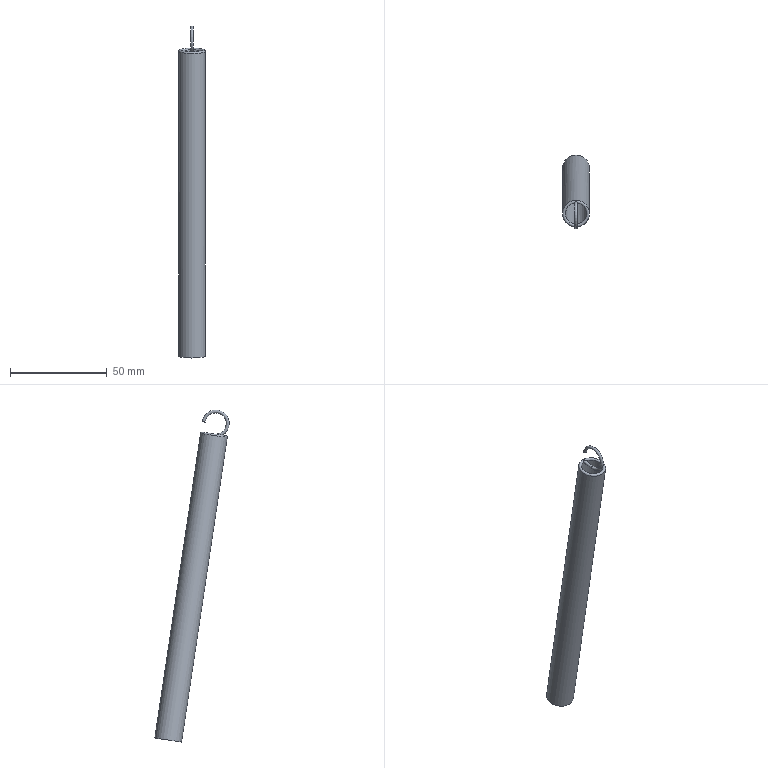Part | NX | features 1 2 | 1 solid | 7 faces | box 14 x 38.473 x 171.94 mm | volume 9491 mm3 | cylinder 3 | plane 2 | torus 2 | commonest cylinder face diameters 1.5 x1 11 x1 14 x1
STEP:
#1=CARTESIAN_POINT('',(-80.065,100.627,-645.601));
#2=VERTEX_POINT('',#1);
#3=CARTESIAN_POINT('',(-80.065,101.371,-645.503));
#4=DIRECTION('',(0.,0.1309,-0.9914));
#5=DIRECTION('',(0.,-0.9914,-0.1309));
#6=AXIS2_PLACEMENT_3D('',#3,#4,#5);
#7=CIRCLE('',#6,0.75);
#8=EDGE_CURVE('',#2,#2,#7,.F.);
#9=ORIENTED_EDGE('',*,*,#8,.F.);
#10=EDGE_LOOP('',(#9));
#11=FACE_BOUND('',#10,.T.);
#12=CARTESIAN_POINT('',(-80.065,101.371,-645.503));
#13=DIRECTION('',(0.,0.1309,-0.9914));
#14=DIRECTION('',(0.,0.9914,0.1309));
#15=AXIS2_PLACEMENT_3D('',#12,#13,#14);
#16=PLANE('',#15);
#17=ADVANCED_FACE('',(#11),#16,.T.);
#18=CARTESIAN_POINT('',(-79.315,96.1,-652.502));
#19=VERTEX_POINT('',#18);
#20=CARTESIAN_POINT('',(-80.065,96.1,-652.502));
#21=DIRECTION('',(0.,0.989,0.1481));
#22=DIRECTION('',(1.,0.,0.));
#23=AXIS2_PLACEMENT_3D('',#20,#21,#22);
#24=CIRCLE('',#23,0.75);
#25=EDGE_CURVE('',#19,#19,#24,.T.);
#26=ORIENTED_EDGE('',*,*,#25,.F.);
#27=EDGE_LOOP('',(#26));
#28=FACE_BOUND('',#27,.T.);
#29=ORIENTED_EDGE('',*,*,#8,.T.);
#30=EDGE_LOOP('',(#29));
#31=FACE_BOUND('',#30,.T.);
#32=CARTESIAN_POINT('',(-80.065,95.174,-646.321));
#33=DIRECTION('',(1.,0.,0.));
#34=DIRECTION('',(0.,-0.989,-0.1481));
#35=AXIS2_PLACEMENT_3D('',#32,#33,#34);
#36=TOROIDAL_SURFACE('',#35,6.25,0.75);
#37=ADVANCED_FACE('',(#28,#31),#36,.T.);
#38=CARTESIAN_POINT('',(-80.065,112.802,-811.261));
#39=VERTEX_POINT('',#38);
#40=CARTESIAN_POINT('',(-80.065,119.725,-810.224));
#41=DIRECTION('',(0.,-0.1481,0.989));
#42=DIRECTION('',(0.,-0.989,-0.1481));
#43=AXIS2_PLACEMENT_3D('',#40,#41,#42);
#44=CIRCLE('',#43,7.);
#45=EDGE_CURVE('',#39,#39,#44,.T.);
#46=ORIENTED_EDGE('',*,*,#45,.T.);
#47=EDGE_LOOP('',(#46));
#48=FACE_BOUND('',#47,.T.);
#49=CARTESIAN_POINT('',(-73.065,96.1,-652.502));
#50=VERTEX_POINT('',#49);
#51=CARTESIAN_POINT('',(-80.065,96.1,-652.502));
#52=DIRECTION('',(0.,0.1481,-0.989));
#53=DIRECTION('',(1.,0.,0.));
#54=AXIS2_PLACEMENT_3D('',#51,#52,#53);
#55=CIRCLE('',#54,7.);
#56=EDGE_CURVE('',#50,#50,#55,.T.);
#57=ORIENTED_EDGE('',*,*,#56,.T.);
#58=EDGE_LOOP('',(#57));
#59=FACE_BOUND('',#58,.T.);
#60=CARTESIAN_POINT('',(-80.065,101.766,-690.33));
#61=DIRECTION('',(0.,0.1481,-0.989));
#62=DIRECTION('',(-1.,0.,0.));
#63=AXIS2_PLACEMENT_3D('',#60,#61,#62);
#64=CYLINDRICAL_SURFACE('',#63,7.);
#65=ADVANCED_FACE('',(#48,#59),#64,.T.);
#66=ORIENTED_EDGE('',*,*,#56,.F.);
#67=EDGE_LOOP('',(#66));
#68=FACE_BOUND('',#67,.T.);
#69=CARTESIAN_POINT('',(-79.315,101.489,-651.695));
#70=VERTEX_POINT('',#69);
#71=CARTESIAN_POINT('',(-80.815,101.489,-651.695));
#72=VERTEX_POINT('',#71);
#73=CARTESIAN_POINT('',(-80.065,96.1,-652.502));
#74=DIRECTION('',(0.,0.1481,-0.989));
#75=DIRECTION('',(-1.,0.,0.));
#76=AXIS2_PLACEMENT_3D('',#73,#74,#75);
#77=CIRCLE('',#76,5.5);
#78=EDGE_CURVE('',#70,#72,#77,.T.);
#79=ORIENTED_EDGE('',*,*,#78,.T.);
#80=CARTESIAN_POINT('',(-80.065,102.17,-650.834));
#81=VERTEX_POINT('',#80);
#82=CARTESIAN_POINT('',(-80.815,101.489,-651.695));
#83=CARTESIAN_POINT('',(-80.815,101.452,-651.451));
#84=CARTESIAN_POINT('',(-80.572,101.669,-651.013));
#85=CARTESIAN_POINT('',(-80.237,102.001,-650.86));
#86=CARTESIAN_POINT('',(-80.065,102.17,-650.834));
#87=B_SPLINE_CURVE_WITH_KNOTS('',3,(#82,#83,#84,#85,#86),.UNSPECIFIED.,.F.,.F.,(4,1,4),(0.,0.0007272,0.001454),.UNSPECIFIED.);
#88=EDGE_CURVE('',#72,#81,#87,.T.);
#89=ORIENTED_EDGE('',*,*,#88,.T.);
#90=CARTESIAN_POINT('',(-79.315,101.489,-651.695));
#91=CARTESIAN_POINT('',(-79.315,101.453,-651.453));
#92=CARTESIAN_POINT('',(-79.56,101.67,-651.011));
#93=CARTESIAN_POINT('',(-79.893,102.,-650.86));
#94=CARTESIAN_POINT('',(-80.065,102.17,-650.834));
#95=B_SPLINE_CURVE_WITH_KNOTS('',3,(#90,#91,#92,#93,#94),.UNSPECIFIED.,.F.,.F.,(4,1,4),(0.0004363,0.001167,0.001898),.UNSPECIFIED.);
#96=EDGE_CURVE('',#81,#70,#95,.F.);
#97=ORIENTED_EDGE('',*,*,#96,.T.);
#98=EDGE_LOOP('',(#79,#89,#97));
#99=FACE_BOUND('',#98,.T.);
#100=CARTESIAN_POINT('',(-80.065,96.1,-652.502));
#101=DIRECTION('',(0.,-0.1481,0.989));
#102=DIRECTION('',(-1.,0.,0.));
#103=AXIS2_PLACEMENT_3D('',#100,#101,#102);
#104=TOROIDAL_SURFACE('',#103,6.25,0.75);
#105=ADVANCED_FACE('',(#68,#99),#104,.T.);
#106=CARTESIAN_POINT('',(-80.815,101.489,-651.695));
#107=CARTESIAN_POINT('',(-80.815,101.548,-652.087));
#108=CARTESIAN_POINT('',(-80.066,101.754,-652.771));
#109=CARTESIAN_POINT('',(-79.315,101.548,-652.087));
#110=CARTESIAN_POINT('',(-79.315,101.489,-651.695));
#111=B_SPLINE_CURVE_WITH_KNOTS('',3,(#106,#107,#108,#109,#110),.UNSPECIFIED.,.F.,.F.,(4,1,4),(0.,0.001174,0.002347),.UNSPECIFIED.);
#112=EDGE_CURVE('',#72,#70,#111,.T.);
#113=ORIENTED_EDGE('',*,*,#112,.T.);
#114=ORIENTED_EDGE('',*,*,#96,.F.);
#115=ORIENTED_EDGE('',*,*,#88,.F.);
#116=EDGE_LOOP('',(#113,#114,#115));
#117=FACE_BOUND('',#116,.T.);
#118=ORIENTED_EDGE('',*,*,#25,.T.);
#119=EDGE_LOOP('',(#118));
#120=FACE_BOUND('',#119,.T.);
#121=CARTESIAN_POINT('',(-80.065,99.191,-652.039));
#122=DIRECTION('',(0.,0.989,0.1481));
#123=DIRECTION('',(-1.,0.,0.));
#124=AXIS2_PLACEMENT_3D('',#121,#122,#123);
#125=CYLINDRICAL_SURFACE('',#124,0.75);
#126=ADVANCED_FACE('',(#117,#120),#125,.T.);
#127=CARTESIAN_POINT('',(-80.065,114.285,-811.038));
#128=VERTEX_POINT('',#127);
#129=CARTESIAN_POINT('',(-80.065,119.725,-810.224));
#130=DIRECTION('',(0.,-0.1481,0.989));
#131=DIRECTION('',(0.,-0.989,-0.1481));
#132=AXIS2_PLACEMENT_3D('',#129,#130,#131);
#133=CIRCLE('',#132,5.5);
#134=EDGE_CURVE('',#128,#128,#133,.F.);
#135=ORIENTED_EDGE('',*,*,#134,.T.);
#136=EDGE_LOOP('',(#135));
#137=FACE_BOUND('',#136,.T.);
#138=ORIENTED_EDGE('',*,*,#112,.F.);
#139=ORIENTED_EDGE('',*,*,#78,.F.);
#140=EDGE_LOOP('',(#138,#139));
#141=FACE_BOUND('',#140,.T.);
#142=CARTESIAN_POINT('',(-80.065,101.766,-690.33));
#143=DIRECTION('',(0.,0.1481,-0.989));
#144=DIRECTION('',(-1.,0.,0.));
#145=AXIS2_PLACEMENT_3D('',#142,#143,#144);
#146=CYLINDRICAL_SURFACE('',#145,5.5);
#147=ADVANCED_FACE('',(#137,#141),#146,.F.);
#148=ORIENTED_EDGE('',*,*,#45,.F.);
#149=EDGE_LOOP('',(#148));
#150=FACE_BOUND('',#149,.T.);
#151=ORIENTED_EDGE('',*,*,#134,.F.);
#152=EDGE_LOOP('',(#151));
#153=FACE_BOUND('',#152,.T.);
#154=CARTESIAN_POINT('',(-80.065,119.725,-810.224));
#155=DIRECTION('',(0.,-0.1481,0.989));
#156=DIRECTION('',(0.,-0.989,-0.1481));
#157=AXIS2_PLACEMENT_3D('',#154,#155,#156);
#158=PLANE('',#157);
#159=ADVANCED_FACE('',(#150,#153),#158,.F.);
#160=CLOSED_SHELL('',(#17,#37,#65,#105,#126,#147,#159));
#161=MANIFOLD_SOLID_BREP('',#160);
#162=(LENGTH_UNIT()NAMED_UNIT(*)SI_UNIT(.MILLI.,.METRE.));
#163=UNCERTAINTY_MEASURE_WITH_UNIT(LENGTH_MEASURE(0.0508),#162,'','');
#164=(NAMED_UNIT(*)PLANE_ANGLE_UNIT()SI_UNIT($,.RADIAN.));
#165=(NAMED_UNIT(*)SI_UNIT($,.STERADIAN.)SOLID_ANGLE_UNIT());
#166=(GEOMETRIC_REPRESENTATION_CONTEXT(3)GLOBAL_UNCERTAINTY_ASSIGNED_CONTEXT((#163))GLOBAL_UNIT_ASSIGNED_CONTEXT((#162,#164,#165))REPRESENTATION_CONTEXT('',''));
#167=ADVANCED_BREP_SHAPE_REPRESENTATION('',(#161),#166);